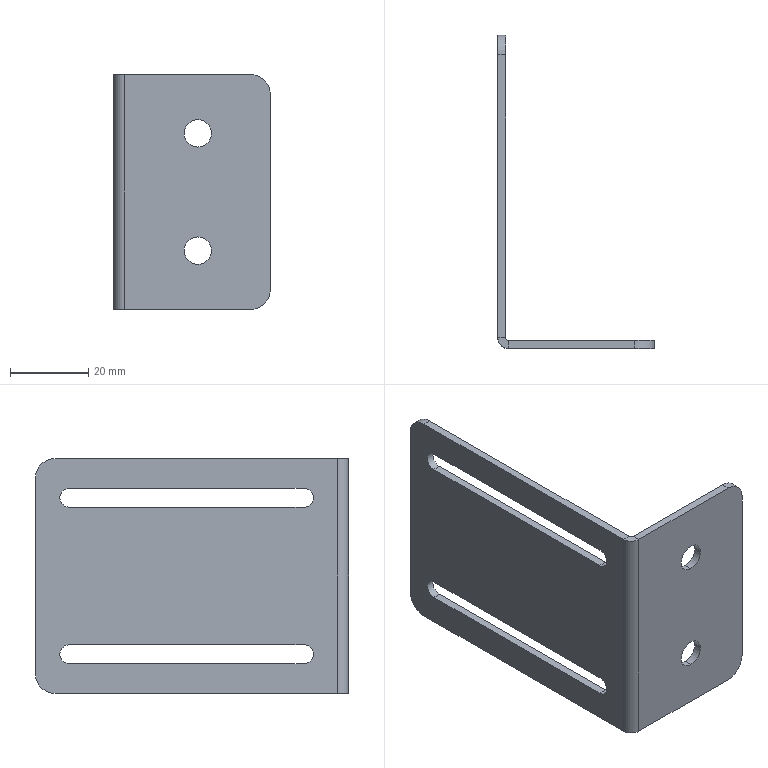Part | SolidWorks | features HoleWzd 2, BreakCorner 1, FlatPattern 1, SMBaseFlange 1, SheetMetal 1 | 1 solid | 30 faces | box 40 x 80 x 60 mm | volume 12649 mm3 | plane 16 | cylinder 14 | commonest cylinder face diameters 4.8 x4 7 x4 10 x4 1.473 x1 5.473 x1
STEP:
#1=CARTESIAN_POINT('',(21.5,0.,11.5));
#2=VERTEX_POINT('',#1);
#3=CARTESIAN_POINT('',(21.5,0.,18.5));
#4=VERTEX_POINT('',#3);
#5=CARTESIAN_POINT('',(21.5,0.,15.));
#6=DIRECTION('',(0.,1.,0.));
#7=DIRECTION('',(0.,0.,1.));
#8=AXIS2_PLACEMENT_3D('',#5,#6,#7);
#9=CIRCLE('',#8,3.5);
#10=EDGE_CURVE('',#2,#4,#9,.T.);
#11=ORIENTED_EDGE('',*,*,#10,.F.);
#12=CARTESIAN_POINT('',(21.5,2.,11.5));
#13=VERTEX_POINT('',#12);
#14=CARTESIAN_POINT('',(21.5,2.,11.5));
#15=DIRECTION('',(0.,1.,0.));
#16=VECTOR('',#15,1000.);
#17=LINE('',#14,#16);
#18=EDGE_CURVE('',#2,#13,#17,.T.);
#19=ORIENTED_EDGE('',*,*,#18,.T.);
#20=CARTESIAN_POINT('',(21.5,2.,18.5));
#21=VERTEX_POINT('',#20);
#22=CARTESIAN_POINT('',(21.5,2.,15.));
#23=DIRECTION('',(0.,1.,0.));
#24=DIRECTION('',(0.,0.,1.));
#25=AXIS2_PLACEMENT_3D('',#22,#23,#24);
#26=CIRCLE('',#25,3.5);
#27=EDGE_CURVE('',#13,#21,#26,.T.);
#28=ORIENTED_EDGE('',*,*,#27,.T.);
#29=CARTESIAN_POINT('',(21.5,2.,18.5));
#30=DIRECTION('',(0.,1.,0.));
#31=VECTOR('',#30,1000.);
#32=LINE('',#29,#31);
#33=EDGE_CURVE('',#4,#21,#32,.T.);
#34=ORIENTED_EDGE('',*,*,#33,.F.);
#35=EDGE_LOOP('',(#11,#19,#28,#34));
#36=FACE_OUTER_BOUND('',#35,.T.);
#37=CARTESIAN_POINT('',(21.5,2.,15.));
#38=DIRECTION('',(0.,1.,0.));
#39=DIRECTION('',(0.,0.,1.));
#40=AXIS2_PLACEMENT_3D('',#37,#38,#39);
#41=CYLINDRICAL_SURFACE('',#40,3.5);
#42=ADVANCED_FACE('',(#36),#41,.F.);
#43=CARTESIAN_POINT('',(21.5,0.,41.5));
#44=VERTEX_POINT('',#43);
#45=CARTESIAN_POINT('',(21.5,0.,48.5));
#46=VERTEX_POINT('',#45);
#47=CARTESIAN_POINT('',(21.5,0.,45.));
#48=DIRECTION('',(0.,1.,0.));
#49=DIRECTION('',(0.,0.,1.));
#50=AXIS2_PLACEMENT_3D('',#47,#48,#49);
#51=CIRCLE('',#50,3.5);
#52=EDGE_CURVE('',#44,#46,#51,.T.);
#53=ORIENTED_EDGE('',*,*,#52,.F.);
#54=CARTESIAN_POINT('',(21.5,2.,41.5));
#55=VERTEX_POINT('',#54);
#56=CARTESIAN_POINT('',(21.5,2.,41.5));
#57=DIRECTION('',(0.,1.,0.));
#58=VECTOR('',#57,1000.);
#59=LINE('',#56,#58);
#60=EDGE_CURVE('',#44,#55,#59,.T.);
#61=ORIENTED_EDGE('',*,*,#60,.T.);
#62=CARTESIAN_POINT('',(21.5,2.,48.5));
#63=VERTEX_POINT('',#62);
#64=CARTESIAN_POINT('',(21.5,2.,45.));
#65=DIRECTION('',(0.,1.,0.));
#66=DIRECTION('',(0.,0.,1.));
#67=AXIS2_PLACEMENT_3D('',#64,#65,#66);
#68=CIRCLE('',#67,3.5);
#69=EDGE_CURVE('',#55,#63,#68,.T.);
#70=ORIENTED_EDGE('',*,*,#69,.T.);
#71=CARTESIAN_POINT('',(21.5,2.,48.5));
#72=DIRECTION('',(0.,1.,0.));
#73=VECTOR('',#72,1000.);
#74=LINE('',#71,#73);
#75=EDGE_CURVE('',#46,#63,#74,.T.);
#76=ORIENTED_EDGE('',*,*,#75,.F.);
#77=EDGE_LOOP('',(#53,#61,#70,#76));
#78=FACE_OUTER_BOUND('',#77,.T.);
#79=CARTESIAN_POINT('',(21.5,2.,45.));
#80=DIRECTION('',(0.,1.,0.));
#81=DIRECTION('',(0.,0.,1.));
#82=AXIS2_PLACEMENT_3D('',#79,#80,#81);
#83=CYLINDRICAL_SURFACE('',#82,3.5);
#84=ADVANCED_FACE('',(#78),#83,.F.);
#85=CARTESIAN_POINT('',(2.,11.368,52.4));
#86=VERTEX_POINT('',#85);
#87=CARTESIAN_POINT('',(2.,11.368,47.6));
#88=VERTEX_POINT('',#87);
#89=CARTESIAN_POINT('',(2.,11.368,50.));
#90=DIRECTION('',(1.,0.,0.));
#91=DIRECTION('',(0.,0.,-1.));
#92=AXIS2_PLACEMENT_3D('',#89,#90,#91);
#93=CIRCLE('',#92,2.4);
#94=EDGE_CURVE('',#86,#88,#93,.T.);
#95=ORIENTED_EDGE('',*,*,#94,.F.);
#96=CARTESIAN_POINT('',(2.,71.368,52.4));
#97=VERTEX_POINT('',#96);
#98=CARTESIAN_POINT('',(2.,11.368,52.4));
#99=DIRECTION('',(0.,1.,0.));
#100=VECTOR('',#99,1000.);
#101=LINE('',#98,#100);
#102=EDGE_CURVE('',#86,#97,#101,.T.);
#103=ORIENTED_EDGE('',*,*,#102,.T.);
#104=CARTESIAN_POINT('',(2.,71.368,47.6));
#105=VERTEX_POINT('',#104);
#106=CARTESIAN_POINT('',(2.,71.368,50.));
#107=DIRECTION('',(1.,0.,0.));
#108=DIRECTION('',(0.,0.,-1.));
#109=AXIS2_PLACEMENT_3D('',#106,#107,#108);
#110=CIRCLE('',#109,2.4);
#111=EDGE_CURVE('',#105,#97,#110,.T.);
#112=ORIENTED_EDGE('',*,*,#111,.F.);
#113=CARTESIAN_POINT('',(2.,11.368,47.6));
#114=DIRECTION('',(0.,1.,0.));
#115=VECTOR('',#114,1000.);
#116=LINE('',#113,#115);
#117=EDGE_CURVE('',#88,#105,#116,.T.);
#118=ORIENTED_EDGE('',*,*,#117,.F.);
#119=EDGE_LOOP('',(#95,#103,#112,#118));
#120=FACE_BOUND('',#119,.T.);
#121=CARTESIAN_POINT('',(2.,80.,55.));
#122=VERTEX_POINT('',#121);
#123=CARTESIAN_POINT('',(2.,80.,5.));
#124=VERTEX_POINT('',#123);
#125=CARTESIAN_POINT('',(2.,80.,60.));
#126=DIRECTION('',(0.,0.,-1.));
#127=VECTOR('',#126,1000.);
#128=LINE('',#125,#127);
#129=EDGE_CURVE('',#122,#124,#128,.T.);
#130=ORIENTED_EDGE('',*,*,#129,.F.);
#131=CARTESIAN_POINT('',(2.,75.,60.));
#132=VERTEX_POINT('',#131);
#133=CARTESIAN_POINT('',(2.,75.,55.));
#134=DIRECTION('',(1.,0.,0.));
#135=DIRECTION('',(0.,0.,1.));
#136=AXIS2_PLACEMENT_3D('',#133,#134,#135);
#137=CIRCLE('',#136,5.);
#138=EDGE_CURVE('',#122,#132,#137,.T.);
#139=ORIENTED_EDGE('',*,*,#138,.T.);
#140=CARTESIAN_POINT('',(2.,2.737,60.));
#141=VERTEX_POINT('',#140);
#142=CARTESIAN_POINT('',(2.,0.,60.));
#143=DIRECTION('',(0.,1.,0.));
#144=VECTOR('',#143,1000.);
#145=LINE('',#142,#144);
#146=EDGE_CURVE('',#141,#132,#145,.T.);
#147=ORIENTED_EDGE('',*,*,#146,.F.);
#148=CARTESIAN_POINT('',(2.,2.737,0.));
#149=VERTEX_POINT('',#148);
#150=CARTESIAN_POINT('',(2.,2.737,60.));
#151=DIRECTION('',(0.,0.,-1.));
#152=VECTOR('',#151,1000.);
#153=LINE('',#150,#152);
#154=EDGE_CURVE('',#141,#149,#153,.T.);
#155=ORIENTED_EDGE('',*,*,#154,.T.);
#156=CARTESIAN_POINT('',(2.,75.,0.));
#157=VERTEX_POINT('',#156);
#158=CARTESIAN_POINT('',(2.,0.,0.));
#159=DIRECTION('',(0.,1.,0.));
#160=VECTOR('',#159,1000.);
#161=LINE('',#158,#160);
#162=EDGE_CURVE('',#149,#157,#161,.T.);
#163=ORIENTED_EDGE('',*,*,#162,.T.);
#164=CARTESIAN_POINT('',(2.,75.,5.));
#165=DIRECTION('',(1.,0.,0.));
#166=DIRECTION('',(0.,0.,1.));
#167=AXIS2_PLACEMENT_3D('',#164,#165,#166);
#168=CIRCLE('',#167,5.);
#169=EDGE_CURVE('',#157,#124,#168,.T.);
#170=ORIENTED_EDGE('',*,*,#169,.T.);
#171=EDGE_LOOP('',(#130,#139,#147,#155,#163,#170));
#172=FACE_OUTER_BOUND('',#171,.T.);
#173=CARTESIAN_POINT('',(2.,11.368,7.6));
#174=VERTEX_POINT('',#173);
#175=CARTESIAN_POINT('',(2.,71.368,7.6));
#176=VERTEX_POINT('',#175);
#177=CARTESIAN_POINT('',(2.,11.368,7.6));
#178=DIRECTION('',(0.,1.,0.));
#179=VECTOR('',#178,1000.);
#180=LINE('',#177,#179);
#181=EDGE_CURVE('',#174,#176,#180,.T.);
#182=ORIENTED_EDGE('',*,*,#181,.F.);
#183=CARTESIAN_POINT('',(2.,11.368,12.4));
#184=VERTEX_POINT('',#183);
#185=CARTESIAN_POINT('',(2.,11.368,10.));
#186=DIRECTION('',(1.,0.,0.));
#187=DIRECTION('',(0.,0.,-1.));
#188=AXIS2_PLACEMENT_3D('',#185,#186,#187);
#189=CIRCLE('',#188,2.4);
#190=EDGE_CURVE('',#184,#174,#189,.T.);
#191=ORIENTED_EDGE('',*,*,#190,.F.);
#192=CARTESIAN_POINT('',(2.,71.368,12.4));
#193=VERTEX_POINT('',#192);
#194=CARTESIAN_POINT('',(2.,11.368,12.4));
#195=DIRECTION('',(0.,1.,0.));
#196=VECTOR('',#195,1000.);
#197=LINE('',#194,#196);
#198=EDGE_CURVE('',#184,#193,#197,.T.);
#199=ORIENTED_EDGE('',*,*,#198,.T.);
#200=CARTESIAN_POINT('',(2.,71.368,10.));
#201=DIRECTION('',(1.,0.,0.));
#202=DIRECTION('',(0.,0.,-1.));
#203=AXIS2_PLACEMENT_3D('',#200,#201,#202);
#204=CIRCLE('',#203,2.4);
#205=EDGE_CURVE('',#176,#193,#204,.T.);
#206=ORIENTED_EDGE('',*,*,#205,.F.);
#207=EDGE_LOOP('',(#182,#191,#199,#206));
#208=FACE_BOUND('',#207,.T.);
#209=CARTESIAN_POINT('',(2.,0.,60.));
#210=DIRECTION('',(-1.,0.,0.));
#211=DIRECTION('',(0.,0.,1.));
#212=AXIS2_PLACEMENT_3D('',#209,#210,#211);
#213=PLANE('',#212);
#214=ADVANCED_FACE('',(#120,#172,#208),#213,.F.);
#215=CARTESIAN_POINT('',(0.,2.737,60.));
#216=VERTEX_POINT('',#215);
#217=CARTESIAN_POINT('',(0.,2.737,60.));
#218=DIRECTION('',(1.,0.,0.));
#219=VECTOR('',#218,1000.);
#220=LINE('',#217,#219);
#221=EDGE_CURVE('',#216,#141,#220,.T.);
#222=ORIENTED_EDGE('',*,*,#221,.F.);
#223=CARTESIAN_POINT('',(2.737,0.,60.));
#224=VERTEX_POINT('',#223);
#225=CARTESIAN_POINT('',(2.737,2.737,60.));
#226=DIRECTION('',(0.,0.,-1.));
#227=DIRECTION('',(1.,0.,0.));
#228=AXIS2_PLACEMENT_3D('',#225,#226,#227);
#229=CIRCLE('',#228,2.737);
#230=EDGE_CURVE('',#224,#216,#229,.T.);
#231=ORIENTED_EDGE('',*,*,#230,.F.);
#232=CARTESIAN_POINT('',(2.737,2.,60.));
#233=VERTEX_POINT('',#232);
#234=CARTESIAN_POINT('',(2.737,2.,60.));
#235=DIRECTION('',(0.,-1.,0.));
#236=VECTOR('',#235,1000.);
#237=LINE('',#234,#236);
#238=EDGE_CURVE('',#233,#224,#237,.T.);
#239=ORIENTED_EDGE('',*,*,#238,.F.);
#240=CARTESIAN_POINT('',(2.737,2.737,60.));
#241=DIRECTION('',(0.,0.,-1.));
#242=DIRECTION('',(1.,0.,0.));
#243=AXIS2_PLACEMENT_3D('',#240,#241,#242);
#244=CIRCLE('',#243,0.7366);
#245=EDGE_CURVE('',#233,#141,#244,.T.);
#246=ORIENTED_EDGE('',*,*,#245,.T.);
#247=EDGE_LOOP('',(#222,#231,#239,#246));
#248=FACE_OUTER_BOUND('',#247,.T.);
#249=CARTESIAN_POINT('',(0.,2.737,60.));
#250=DIRECTION('',(0.,0.,1.));
#251=DIRECTION('',(1.,0.,0.));
#252=AXIS2_PLACEMENT_3D('',#249,#250,#251);
#253=PLANE('',#252);
#254=ADVANCED_FACE('',(#248),#253,.T.);
#255=ORIENTED_EDGE('',*,*,#146,.T.);
#256=CARTESIAN_POINT('',(0.,75.,60.));
#257=VERTEX_POINT('',#256);
#258=CARTESIAN_POINT('',(2.737,75.,60.));
#259=DIRECTION('',(-1.,0.,0.));
#260=VECTOR('',#259,1000.);
#261=LINE('',#258,#260);
#262=EDGE_CURVE('',#132,#257,#261,.T.);
#263=ORIENTED_EDGE('',*,*,#262,.T.);
#264=CARTESIAN_POINT('',(0.,0.,60.));
#265=DIRECTION('',(0.,1.,0.));
#266=VECTOR('',#265,1000.);
#267=LINE('',#264,#266);
#268=EDGE_CURVE('',#216,#257,#267,.T.);
#269=ORIENTED_EDGE('',*,*,#268,.F.);
#270=ORIENTED_EDGE('',*,*,#221,.T.);
#271=EDGE_LOOP('',(#255,#263,#269,#270));
#272=FACE_OUTER_BOUND('',#271,.T.);
#273=CARTESIAN_POINT('',(2.737,2.,60.));
#274=DIRECTION('',(0.,0.,1.));
#275=DIRECTION('',(1.,0.,0.));
#276=AXIS2_PLACEMENT_3D('',#273,#274,#275);
#277=PLANE('',#276);
#278=ADVANCED_FACE('',(#272),#277,.T.);
#279=CARTESIAN_POINT('',(2.737,0.,0.));
#280=VERTEX_POINT('',#279);
#281=CARTESIAN_POINT('',(2.737,2.,0.));
#282=VERTEX_POINT('',#281);
#283=CARTESIAN_POINT('',(2.737,0.,0.));
#284=DIRECTION('',(0.,1.,0.));
#285=VECTOR('',#284,1000.);
#286=LINE('',#283,#285);
#287=EDGE_CURVE('',#280,#282,#286,.T.);
#288=ORIENTED_EDGE('',*,*,#287,.F.);
#289=CARTESIAN_POINT('',(0.,2.737,0.));
#290=VERTEX_POINT('',#289);
#291=CARTESIAN_POINT('',(2.737,2.737,0.));
#292=DIRECTION('',(0.,0.,-1.));
#293=DIRECTION('',(1.,0.,0.));
#294=AXIS2_PLACEMENT_3D('',#291,#292,#293);
#295=CIRCLE('',#294,2.737);
#296=EDGE_CURVE('',#280,#290,#295,.T.);
#297=ORIENTED_EDGE('',*,*,#296,.T.);
#298=CARTESIAN_POINT('',(2.,2.737,0.));
#299=DIRECTION('',(-1.,0.,0.));
#300=VECTOR('',#299,1000.);
#301=LINE('',#298,#300);
#302=EDGE_CURVE('',#149,#290,#301,.T.);
#303=ORIENTED_EDGE('',*,*,#302,.F.);
#304=CARTESIAN_POINT('',(2.737,2.737,0.));
#305=DIRECTION('',(0.,0.,-1.));
#306=DIRECTION('',(1.,0.,0.));
#307=AXIS2_PLACEMENT_3D('',#304,#305,#306);
#308=CIRCLE('',#307,0.7366);
#309=EDGE_CURVE('',#282,#149,#308,.T.);
#310=ORIENTED_EDGE('',*,*,#309,.F.);
#311=EDGE_LOOP('',(#288,#297,#303,#310));
#312=FACE_OUTER_BOUND('',#311,.T.);
#313=CARTESIAN_POINT('',(2.737,0.,0.));
#314=DIRECTION('',(0.,0.,-1.));
#315=DIRECTION('',(-1.,0.,0.));
#316=AXIS2_PLACEMENT_3D('',#313,#314,#315);
#317=PLANE('',#316);
#318=ADVANCED_FACE('',(#312),#317,.T.);
#319=CARTESIAN_POINT('',(35.,2.,0.));
#320=VERTEX_POINT('',#319);
#321=CARTESIAN_POINT('',(0.,2.,0.));
#322=DIRECTION('',(-1.,0.,0.));
#323=VECTOR('',#322,1000.);
#324=LINE('',#321,#323);
#325=EDGE_CURVE('',#320,#282,#324,.T.);
#326=ORIENTED_EDGE('',*,*,#325,.F.);
#327=CARTESIAN_POINT('',(35.,0.,0.));
#328=VERTEX_POINT('',#327);
#329=CARTESIAN_POINT('',(35.,2.737,0.));
#330=DIRECTION('',(0.,-1.,0.));
#331=VECTOR('',#330,1000.);
#332=LINE('',#329,#331);
#333=EDGE_CURVE('',#320,#328,#332,.T.);
#334=ORIENTED_EDGE('',*,*,#333,.T.);
#335=CARTESIAN_POINT('',(0.,0.,0.));
#336=DIRECTION('',(-1.,0.,0.));
#337=VECTOR('',#336,1000.);
#338=LINE('',#335,#337);
#339=EDGE_CURVE('',#328,#280,#338,.T.);
#340=ORIENTED_EDGE('',*,*,#339,.T.);
#341=ORIENTED_EDGE('',*,*,#287,.T.);
#342=EDGE_LOOP('',(#326,#334,#340,#341));
#343=FACE_OUTER_BOUND('',#342,.T.);
#344=CARTESIAN_POINT('',(2.,2.737,0.));
#345=DIRECTION('',(0.,0.,-1.));
#346=DIRECTION('',(-1.,0.,0.));
#347=AXIS2_PLACEMENT_3D('',#344,#345,#346);
#348=PLANE('',#347);
#349=ADVANCED_FACE('',(#343),#348,.T.);
#350=CARTESIAN_POINT('',(0.,80.,55.));
#351=VERTEX_POINT('',#350);
#352=CARTESIAN_POINT('',(0.,80.,5.));
#353=VERTEX_POINT('',#352);
#354=CARTESIAN_POINT('',(0.,80.,60.));
#355=DIRECTION('',(0.,0.,-1.));
#356=VECTOR('',#355,1000.);
#357=LINE('',#354,#356);
#358=EDGE_CURVE('',#351,#353,#357,.T.);
#359=ORIENTED_EDGE('',*,*,#358,.F.);
#360=CARTESIAN_POINT('',(0.,80.,55.));
#361=DIRECTION('',(1.,0.,0.));
#362=VECTOR('',#361,1000.);
#363=LINE('',#360,#362);
#364=EDGE_CURVE('',#351,#122,#363,.T.);
#365=ORIENTED_EDGE('',*,*,#364,.T.);
#366=ORIENTED_EDGE('',*,*,#129,.T.);
#367=CARTESIAN_POINT('',(0.,80.,5.));
#368=DIRECTION('',(-1.,0.,0.));
#369=VECTOR('',#368,1000.);
#370=LINE('',#367,#369);
#371=EDGE_CURVE('',#124,#353,#370,.T.);
#372=ORIENTED_EDGE('',*,*,#371,.T.);
#373=EDGE_LOOP('',(#359,#365,#366,#372));
#374=FACE_OUTER_BOUND('',#373,.T.);
#375=CARTESIAN_POINT('',(0.,80.,60.));
#376=DIRECTION('',(0.,1.,0.));
#377=DIRECTION('',(0.,0.,1.));
#378=AXIS2_PLACEMENT_3D('',#375,#376,#377);
#379=PLANE('',#378);
#380=ADVANCED_FACE('',(#374),#379,.T.);
#381=CARTESIAN_POINT('',(0.,11.368,52.4));
#382=VERTEX_POINT('',#381);
#383=CARTESIAN_POINT('',(0.,71.368,52.4));
#384=VERTEX_POINT('',#383);
#385=CARTESIAN_POINT('',(0.,11.368,52.4));
#386=DIRECTION('',(0.,1.,0.));
#387=VECTOR('',#386,1000.);
#388=LINE('',#385,#387);
#389=EDGE_CURVE('',#382,#384,#388,.T.);
#390=ORIENTED_EDGE('',*,*,#389,.F.);
#391=CARTESIAN_POINT('',(0.,11.368,47.6));
#392=VERTEX_POINT('',#391);
#393=CARTESIAN_POINT('',(0.,11.368,50.));
#394=DIRECTION('',(1.,0.,0.));
#395=DIRECTION('',(0.,0.,-1.));
#396=AXIS2_PLACEMENT_3D('',#393,#394,#395);
#397=CIRCLE('',#396,2.4);
#398=EDGE_CURVE('',#382,#392,#397,.T.);
#399=ORIENTED_EDGE('',*,*,#398,.T.);
#400=CARTESIAN_POINT('',(0.,71.368,47.6));
#401=VERTEX_POINT('',#400);
#402=CARTESIAN_POINT('',(0.,11.368,47.6));
#403=DIRECTION('',(0.,1.,0.));
#404=VECTOR('',#403,1000.);
#405=LINE('',#402,#404);
#406=EDGE_CURVE('',#392,#401,#405,.T.);
#407=ORIENTED_EDGE('',*,*,#406,.T.);
#408=CARTESIAN_POINT('',(0.,71.368,50.));
#409=DIRECTION('',(1.,0.,0.));
#410=DIRECTION('',(0.,0.,-1.));
#411=AXIS2_PLACEMENT_3D('',#408,#409,#410);
#412=CIRCLE('',#411,2.4);
#413=EDGE_CURVE('',#401,#384,#412,.T.);
#414=ORIENTED_EDGE('',*,*,#413,.T.);
#415=EDGE_LOOP('',(#390,#399,#407,#414));
#416=FACE_BOUND('',#415,.T.);
#417=CARTESIAN_POINT('',(0.,11.368,12.4));
#418=VERTEX_POINT('',#417);
#419=CARTESIAN_POINT('',(0.,11.368,7.6));
#420=VERTEX_POINT('',#419);
#421=CARTESIAN_POINT('',(0.,11.368,10.));
#422=DIRECTION('',(1.,0.,0.));
#423=DIRECTION('',(0.,0.,-1.));
#424=AXIS2_PLACEMENT_3D('',#421,#422,#423);
#425=CIRCLE('',#424,2.4);
#426=EDGE_CURVE('',#418,#420,#425,.T.);
#427=ORIENTED_EDGE('',*,*,#426,.T.);
#428=CARTESIAN_POINT('',(0.,71.368,7.6));
#429=VERTEX_POINT('',#428);
#430=CARTESIAN_POINT('',(0.,11.368,7.6));
#431=DIRECTION('',(0.,1.,0.));
#432=VECTOR('',#431,1000.);
#433=LINE('',#430,#432);
#434=EDGE_CURVE('',#420,#429,#433,.T.);
#435=ORIENTED_EDGE('',*,*,#434,.T.);
#436=CARTESIAN_POINT('',(0.,71.368,12.4));
#437=VERTEX_POINT('',#436);
#438=CARTESIAN_POINT('',(0.,71.368,10.));
#439=DIRECTION('',(1.,0.,0.));
#440=DIRECTION('',(0.,0.,-1.));
#441=AXIS2_PLACEMENT_3D('',#438,#439,#440);
#442=CIRCLE('',#441,2.4);
#443=EDGE_CURVE('',#429,#437,#442,.T.);
#444=ORIENTED_EDGE('',*,*,#443,.T.);
#445=CARTESIAN_POINT('',(0.,11.368,12.4));
#446=DIRECTION('',(0.,1.,0.));
#447=VECTOR('',#446,1000.);
#448=LINE('',#445,#447);
#449=EDGE_CURVE('',#418,#437,#448,.T.);
#450=ORIENTED_EDGE('',*,*,#449,.F.);
#451=EDGE_LOOP('',(#427,#435,#444,#450));
#452=FACE_BOUND('',#451,.T.);
#453=ORIENTED_EDGE('',*,*,#268,.T.);
#454=CARTESIAN_POINT('',(0.,75.,55.));
#455=DIRECTION('',(-1.,0.,0.));
#456=DIRECTION('',(0.,0.,1.));
#457=AXIS2_PLACEMENT_3D('',#454,#455,#456);
#458=CIRCLE('',#457,5.);
#459=EDGE_CURVE('',#257,#351,#458,.T.);
#460=ORIENTED_EDGE('',*,*,#459,.T.);
#461=ORIENTED_EDGE('',*,*,#358,.T.);
#462=CARTESIAN_POINT('',(0.,75.,0.));
#463=VERTEX_POINT('',#462);
#464=CARTESIAN_POINT('',(0.,75.,5.));
#465=DIRECTION('',(-1.,0.,0.));
#466=DIRECTION('',(0.,0.,1.));
#467=AXIS2_PLACEMENT_3D('',#464,#465,#466);
#468=CIRCLE('',#467,5.);
#469=EDGE_CURVE('',#353,#463,#468,.T.);
#470=ORIENTED_EDGE('',*,*,#469,.T.);
#471=CARTESIAN_POINT('',(0.,0.,0.));
#472=DIRECTION('',(0.,1.,0.));
#473=VECTOR('',#472,1000.);
#474=LINE('',#471,#473);
#475=EDGE_CURVE('',#290,#463,#474,.T.);
#476=ORIENTED_EDGE('',*,*,#475,.F.);
#477=CARTESIAN_POINT('',(0.,2.737,60.));
#478=DIRECTION('',(0.,0.,-1.));
#479=VECTOR('',#478,1000.);
#480=LINE('',#477,#479);
#481=EDGE_CURVE('',#216,#290,#480,.T.);
#482=ORIENTED_EDGE('',*,*,#481,.F.);
#483=EDGE_LOOP('',(#453,#460,#461,#470,#476,#482));
#484=FACE_OUTER_BOUND('',#483,.T.);
#485=CARTESIAN_POINT('',(0.,0.,60.));
#486=DIRECTION('',(-1.,0.,0.));
#487=DIRECTION('',(0.,0.,1.));
#488=AXIS2_PLACEMENT_3D('',#485,#486,#487);
#489=PLANE('',#488);
#490=ADVANCED_FACE('',(#416,#452,#484),#489,.T.);
#491=ORIENTED_EDGE('',*,*,#296,.F.);
#492=CARTESIAN_POINT('',(2.737,0.,60.));
#493=DIRECTION('',(0.,0.,-1.));
#494=VECTOR('',#493,1000.);
#495=LINE('',#492,#494);
#496=EDGE_CURVE('',#224,#280,#495,.T.);
#497=ORIENTED_EDGE('',*,*,#496,.F.);
#498=ORIENTED_EDGE('',*,*,#230,.T.);
#499=ORIENTED_EDGE('',*,*,#481,.T.);
#500=EDGE_LOOP('',(#491,#497,#498,#499));
#501=FACE_OUTER_BOUND('',#500,.T.);
#502=CARTESIAN_POINT('',(2.737,2.737,60.));
#503=DIRECTION('',(0.,0.,-1.));
#504=DIRECTION('',(-1.,0.,0.));
#505=AXIS2_PLACEMENT_3D('',#502,#503,#504);
#506=CYLINDRICAL_SURFACE('',#505,2.737);
#507=ADVANCED_FACE('',(#501),#506,.T.);
#508=CARTESIAN_POINT('',(21.5,0.,15.));
#509=DIRECTION('',(0.,1.,0.));
#510=DIRECTION('',(0.,0.,1.));
#511=AXIS2_PLACEMENT_3D('',#508,#509,#510);
#512=CIRCLE('',#511,3.5);
#513=EDGE_CURVE('',#4,#2,#512,.T.);
#514=ORIENTED_EDGE('',*,*,#513,.T.);
#515=ORIENTED_EDGE('',*,*,#10,.T.);
#516=EDGE_LOOP('',(#514,#515));
#517=FACE_BOUND('',#516,.T.);
#518=CARTESIAN_POINT('',(21.5,0.,45.));
#519=DIRECTION('',(0.,1.,0.));
#520=DIRECTION('',(0.,0.,1.));
#521=AXIS2_PLACEMENT_3D('',#518,#519,#520);
#522=CIRCLE('',#521,3.5);
#523=EDGE_CURVE('',#46,#44,#522,.T.);
#524=ORIENTED_EDGE('',*,*,#523,.T.);
#525=ORIENTED_EDGE('',*,*,#52,.T.);
#526=EDGE_LOOP('',(#524,#525));
#527=FACE_BOUND('',#526,.T.);
#528=CARTESIAN_POINT('',(40.,0.,55.));
#529=VERTEX_POINT('',#528);
#530=CARTESIAN_POINT('',(40.,0.,5.));
#531=VERTEX_POINT('',#530);
#532=CARTESIAN_POINT('',(40.,0.,60.));
#533=DIRECTION('',(0.,0.,-1.));
#534=VECTOR('',#533,1000.);
#535=LINE('',#532,#534);
#536=EDGE_CURVE('',#529,#531,#535,.T.);
#537=ORIENTED_EDGE('',*,*,#536,.F.);
#538=CARTESIAN_POINT('',(35.,0.,60.));
#539=VERTEX_POINT('',#538);
#540=CARTESIAN_POINT('',(35.,0.,55.));
#541=DIRECTION('',(0.,-1.,0.));
#542=DIRECTION('',(0.,0.,-1.));
#543=AXIS2_PLACEMENT_3D('',#540,#541,#542);
#544=CIRCLE('',#543,5.);
#545=EDGE_CURVE('',#529,#539,#544,.T.);
#546=ORIENTED_EDGE('',*,*,#545,.T.);
#547=CARTESIAN_POINT('',(0.,0.,60.));
#548=DIRECTION('',(-1.,0.,0.));
#549=VECTOR('',#548,1000.);
#550=LINE('',#547,#549);
#551=EDGE_CURVE('',#539,#224,#550,.T.);
#552=ORIENTED_EDGE('',*,*,#551,.T.);
#553=ORIENTED_EDGE('',*,*,#496,.T.);
#554=ORIENTED_EDGE('',*,*,#339,.F.);
#555=CARTESIAN_POINT('',(35.,0.,5.));
#556=DIRECTION('',(0.,-1.,0.));
#557=DIRECTION('',(0.,0.,-1.));
#558=AXIS2_PLACEMENT_3D('',#555,#556,#557);
#559=CIRCLE('',#558,5.);
#560=EDGE_CURVE('',#328,#531,#559,.T.);
#561=ORIENTED_EDGE('',*,*,#560,.T.);
#562=EDGE_LOOP('',(#537,#546,#552,#553,#554,#561));
#563=FACE_OUTER_BOUND('',#562,.T.);
#564=CARTESIAN_POINT('',(0.,0.,60.));
#565=DIRECTION('',(0.,-1.,0.));
#566=DIRECTION('',(0.,0.,-1.));
#567=AXIS2_PLACEMENT_3D('',#564,#565,#566);
#568=PLANE('',#567);
#569=ADVANCED_FACE('',(#517,#527,#563),#568,.T.);
#570=CARTESIAN_POINT('',(40.,2.,55.));
#571=VERTEX_POINT('',#570);
#572=CARTESIAN_POINT('',(40.,2.,5.));
#573=VERTEX_POINT('',#572);
#574=CARTESIAN_POINT('',(40.,2.,60.));
#575=DIRECTION('',(0.,0.,-1.));
#576=VECTOR('',#575,1000.);
#577=LINE('',#574,#576);
#578=EDGE_CURVE('',#571,#573,#577,.T.);
#579=ORIENTED_EDGE('',*,*,#578,.F.);
#580=CARTESIAN_POINT('',(40.,2.,55.));
#581=DIRECTION('',(0.,-1.,0.));
#582=VECTOR('',#581,1000.);
#583=LINE('',#580,#582);
#584=EDGE_CURVE('',#571,#529,#583,.T.);
#585=ORIENTED_EDGE('',*,*,#584,.T.);
#586=ORIENTED_EDGE('',*,*,#536,.T.);
#587=CARTESIAN_POINT('',(40.,2.,5.));
#588=DIRECTION('',(0.,1.,0.));
#589=VECTOR('',#588,1000.);
#590=LINE('',#587,#589);
#591=EDGE_CURVE('',#531,#573,#590,.T.);
#592=ORIENTED_EDGE('',*,*,#591,.T.);
#593=EDGE_LOOP('',(#579,#585,#586,#592));
#594=FACE_OUTER_BOUND('',#593,.T.);
#595=CARTESIAN_POINT('',(40.,2.,60.));
#596=DIRECTION('',(1.,0.,0.));
#597=DIRECTION('',(0.,0.,-1.));
#598=AXIS2_PLACEMENT_3D('',#595,#596,#597);
#599=PLANE('',#598);
#600=ADVANCED_FACE('',(#594),#599,.T.);
#601=CARTESIAN_POINT('',(21.5,2.,15.));
#602=DIRECTION('',(0.,1.,0.));
#603=DIRECTION('',(0.,0.,1.));
#604=AXIS2_PLACEMENT_3D('',#601,#602,#603);
#605=CIRCLE('',#604,3.5);
#606=EDGE_CURVE('',#21,#13,#605,.T.);
#607=ORIENTED_EDGE('',*,*,#606,.F.);
#608=ORIENTED_EDGE('',*,*,#27,.F.);
#609=EDGE_LOOP('',(#607,#608));
#610=FACE_BOUND('',#609,.T.);
#611=CARTESIAN_POINT('',(21.5,2.,45.));
#612=DIRECTION('',(0.,1.,0.));
#613=DIRECTION('',(0.,0.,1.));
#614=AXIS2_PLACEMENT_3D('',#611,#612,#613);
#615=CIRCLE('',#614,3.5);
#616=EDGE_CURVE('',#63,#55,#615,.T.);
#617=ORIENTED_EDGE('',*,*,#616,.F.);
#618=ORIENTED_EDGE('',*,*,#69,.F.);
#619=EDGE_LOOP('',(#617,#618));
#620=FACE_BOUND('',#619,.T.);
#621=CARTESIAN_POINT('',(35.,2.,60.));
#622=VERTEX_POINT('',#621);
#623=CARTESIAN_POINT('',(0.,2.,60.));
#624=DIRECTION('',(-1.,0.,0.));
#625=VECTOR('',#624,1000.);
#626=LINE('',#623,#625);
#627=EDGE_CURVE('',#622,#233,#626,.T.);
#628=ORIENTED_EDGE('',*,*,#627,.F.);
#629=CARTESIAN_POINT('',(35.,2.,55.));
#630=DIRECTION('',(0.,1.,0.));
#631=DIRECTION('',(0.,0.,-1.));
#632=AXIS2_PLACEMENT_3D('',#629,#630,#631);
#633=CIRCLE('',#632,5.);
#634=EDGE_CURVE('',#622,#571,#633,.T.);
#635=ORIENTED_EDGE('',*,*,#634,.T.);
#636=ORIENTED_EDGE('',*,*,#578,.T.);
#637=CARTESIAN_POINT('',(35.,2.,5.));
#638=DIRECTION('',(0.,1.,0.));
#639=DIRECTION('',(0.,0.,-1.));
#640=AXIS2_PLACEMENT_3D('',#637,#638,#639);
#641=CIRCLE('',#640,5.);
#642=EDGE_CURVE('',#573,#320,#641,.T.);
#643=ORIENTED_EDGE('',*,*,#642,.T.);
#644=ORIENTED_EDGE('',*,*,#325,.T.);
#645=CARTESIAN_POINT('',(2.737,2.,60.));
#646=DIRECTION('',(0.,0.,-1.));
#647=VECTOR('',#646,1000.);
#648=LINE('',#645,#647);
#649=EDGE_CURVE('',#233,#282,#648,.T.);
#650=ORIENTED_EDGE('',*,*,#649,.F.);
#651=EDGE_LOOP('',(#628,#635,#636,#643,#644,#650));
#652=FACE_OUTER_BOUND('',#651,.T.);
#653=CARTESIAN_POINT('',(0.,2.,60.));
#654=DIRECTION('',(0.,-1.,0.));
#655=DIRECTION('',(0.,0.,-1.));
#656=AXIS2_PLACEMENT_3D('',#653,#654,#655);
#657=PLANE('',#656);
#658=ADVANCED_FACE('',(#610,#620,#652),#657,.F.);
#659=ORIENTED_EDGE('',*,*,#309,.T.);
#660=ORIENTED_EDGE('',*,*,#154,.F.);
#661=ORIENTED_EDGE('',*,*,#245,.F.);
#662=ORIENTED_EDGE('',*,*,#649,.T.);
#663=EDGE_LOOP('',(#659,#660,#661,#662));
#664=FACE_OUTER_BOUND('',#663,.T.);
#665=CARTESIAN_POINT('',(2.737,2.737,60.));
#666=DIRECTION('',(0.,0.,-1.));
#667=DIRECTION('',(-1.,0.,0.));
#668=AXIS2_PLACEMENT_3D('',#665,#666,#667);
#669=CYLINDRICAL_SURFACE('',#668,0.7366);
#670=ADVANCED_FACE('',(#664),#669,.F.);
#671=ORIENTED_EDGE('',*,*,#551,.F.);
#672=CARTESIAN_POINT('',(35.,2.737,60.));
#673=DIRECTION('',(0.,1.,0.));
#674=VECTOR('',#673,1000.);
#675=LINE('',#672,#674);
#676=EDGE_CURVE('',#539,#622,#675,.T.);
#677=ORIENTED_EDGE('',*,*,#676,.T.);
#678=ORIENTED_EDGE('',*,*,#627,.T.);
#679=ORIENTED_EDGE('',*,*,#238,.T.);
#680=EDGE_LOOP('',(#671,#677,#678,#679));
#681=FACE_OUTER_BOUND('',#680,.T.);
#682=CARTESIAN_POINT('',(2.737,2.737,60.));
#683=DIRECTION('',(0.,0.,1.));
#684=DIRECTION('',(1.,0.,0.));
#685=AXIS2_PLACEMENT_3D('',#682,#683,#684);
#686=PLANE('',#685);
#687=ADVANCED_FACE('',(#681),#686,.T.);
#688=ORIENTED_EDGE('',*,*,#475,.T.);
#689=CARTESIAN_POINT('',(2.,75.,0.));
#690=DIRECTION('',(1.,0.,0.));
#691=VECTOR('',#690,1000.);
#692=LINE('',#689,#691);
#693=EDGE_CURVE('',#463,#157,#692,.T.);
#694=ORIENTED_EDGE('',*,*,#693,.T.);
#695=ORIENTED_EDGE('',*,*,#162,.F.);
#696=ORIENTED_EDGE('',*,*,#302,.T.);
#697=EDGE_LOOP('',(#688,#694,#695,#696));
#698=FACE_OUTER_BOUND('',#697,.T.);
#699=CARTESIAN_POINT('',(2.737,2.737,0.));
#700=DIRECTION('',(0.,0.,1.));
#701=DIRECTION('',(1.,0.,0.));
#702=AXIS2_PLACEMENT_3D('',#699,#700,#701);
#703=PLANE('',#702);
#704=ADVANCED_FACE('',(#698),#703,.F.);
#705=ORIENTED_EDGE('',*,*,#443,.F.);
#706=CARTESIAN_POINT('',(2.,71.368,7.6));
#707=DIRECTION('',(-1.,0.,0.));
#708=VECTOR('',#707,1000.);
#709=LINE('',#706,#708);
#710=EDGE_CURVE('',#176,#429,#709,.T.);
#711=ORIENTED_EDGE('',*,*,#710,.F.);
#712=ORIENTED_EDGE('',*,*,#205,.T.);
#713=CARTESIAN_POINT('',(2.,71.368,12.4));
#714=DIRECTION('',(1.,0.,0.));
#715=VECTOR('',#714,1000.);
#716=LINE('',#713,#715);
#717=EDGE_CURVE('',#437,#193,#716,.T.);
#718=ORIENTED_EDGE('',*,*,#717,.F.);
#719=EDGE_LOOP('',(#705,#711,#712,#718));
#720=FACE_OUTER_BOUND('',#719,.T.);
#721=CARTESIAN_POINT('',(2.,71.368,10.));
#722=DIRECTION('',(1.,0.,0.));
#723=DIRECTION('',(0.,0.,-1.));
#724=AXIS2_PLACEMENT_3D('',#721,#722,#723);
#725=CYLINDRICAL_SURFACE('',#724,2.4);
#726=ADVANCED_FACE('',(#720),#725,.F.);
#727=ORIENTED_EDGE('',*,*,#190,.T.);
#728=CARTESIAN_POINT('',(2.,11.368,7.6));
#729=DIRECTION('',(1.,0.,0.));
#730=VECTOR('',#729,1000.);
#731=LINE('',#728,#730);
#732=EDGE_CURVE('',#420,#174,#731,.T.);
#733=ORIENTED_EDGE('',*,*,#732,.F.);
#734=ORIENTED_EDGE('',*,*,#426,.F.);
#735=CARTESIAN_POINT('',(2.,11.368,12.4));
#736=DIRECTION('',(-1.,0.,0.));
#737=VECTOR('',#736,1000.);
#738=LINE('',#735,#737);
#739=EDGE_CURVE('',#184,#418,#738,.T.);
#740=ORIENTED_EDGE('',*,*,#739,.F.);
#741=EDGE_LOOP('',(#727,#733,#734,#740));
#742=FACE_OUTER_BOUND('',#741,.T.);
#743=CARTESIAN_POINT('',(2.,11.368,10.));
#744=DIRECTION('',(1.,0.,0.));
#745=DIRECTION('',(0.,0.,-1.));
#746=AXIS2_PLACEMENT_3D('',#743,#744,#745);
#747=CYLINDRICAL_SURFACE('',#746,2.4);
#748=ADVANCED_FACE('',(#742),#747,.F.);
#749=ORIENTED_EDGE('',*,*,#717,.T.);
#750=ORIENTED_EDGE('',*,*,#198,.F.);
#751=ORIENTED_EDGE('',*,*,#739,.T.);
#752=ORIENTED_EDGE('',*,*,#449,.T.);
#753=EDGE_LOOP('',(#749,#750,#751,#752));
#754=FACE_OUTER_BOUND('',#753,.T.);
#755=CARTESIAN_POINT('',(2.,11.368,12.4));
#756=DIRECTION('',(0.,0.,1.));
#757=DIRECTION('',(1.,0.,0.));
#758=AXIS2_PLACEMENT_3D('',#755,#756,#757);
#759=PLANE('',#758);
#760=ADVANCED_FACE('',(#754),#759,.F.);
#761=ORIENTED_EDGE('',*,*,#710,.T.);
#762=ORIENTED_EDGE('',*,*,#434,.F.);
#763=ORIENTED_EDGE('',*,*,#732,.T.);
#764=ORIENTED_EDGE('',*,*,#181,.T.);
#765=EDGE_LOOP('',(#761,#762,#763,#764));
#766=FACE_OUTER_BOUND('',#765,.T.);
#767=CARTESIAN_POINT('',(2.,11.368,7.6));
#768=DIRECTION('',(0.,0.,-1.));
#769=DIRECTION('',(-1.,0.,0.));
#770=AXIS2_PLACEMENT_3D('',#767,#768,#769);
#771=PLANE('',#770);
#772=ADVANCED_FACE('',(#766),#771,.F.);
#773=ORIENTED_EDGE('',*,*,#413,.F.);
#774=CARTESIAN_POINT('',(2.,71.368,47.6));
#775=DIRECTION('',(-1.,0.,0.));
#776=VECTOR('',#775,1000.);
#777=LINE('',#774,#776);
#778=EDGE_CURVE('',#105,#401,#777,.T.);
#779=ORIENTED_EDGE('',*,*,#778,.F.);
#780=ORIENTED_EDGE('',*,*,#111,.T.);
#781=CARTESIAN_POINT('',(2.,71.368,52.4));
#782=DIRECTION('',(1.,0.,0.));
#783=VECTOR('',#782,1000.);
#784=LINE('',#781,#783);
#785=EDGE_CURVE('',#384,#97,#784,.T.);
#786=ORIENTED_EDGE('',*,*,#785,.F.);
#787=EDGE_LOOP('',(#773,#779,#780,#786));
#788=FACE_OUTER_BOUND('',#787,.T.);
#789=CARTESIAN_POINT('',(2.,71.368,50.));
#790=DIRECTION('',(1.,0.,0.));
#791=DIRECTION('',(0.,0.,-1.));
#792=AXIS2_PLACEMENT_3D('',#789,#790,#791);
#793=CYLINDRICAL_SURFACE('',#792,2.4);
#794=ADVANCED_FACE('',(#788),#793,.F.);
#795=ORIENTED_EDGE('',*,*,#94,.T.);
#796=CARTESIAN_POINT('',(2.,11.368,47.6));
#797=DIRECTION('',(1.,0.,0.));
#798=VECTOR('',#797,1000.);
#799=LINE('',#796,#798);
#800=EDGE_CURVE('',#392,#88,#799,.T.);
#801=ORIENTED_EDGE('',*,*,#800,.F.);
#802=ORIENTED_EDGE('',*,*,#398,.F.);
#803=CARTESIAN_POINT('',(2.,11.368,52.4));
#804=DIRECTION('',(-1.,0.,0.));
#805=VECTOR('',#804,1000.);
#806=LINE('',#803,#805);
#807=EDGE_CURVE('',#86,#382,#806,.T.);
#808=ORIENTED_EDGE('',*,*,#807,.F.);
#809=EDGE_LOOP('',(#795,#801,#802,#808));
#810=FACE_OUTER_BOUND('',#809,.T.);
#811=CARTESIAN_POINT('',(2.,11.368,50.));
#812=DIRECTION('',(1.,0.,0.));
#813=DIRECTION('',(0.,0.,-1.));
#814=AXIS2_PLACEMENT_3D('',#811,#812,#813);
#815=CYLINDRICAL_SURFACE('',#814,2.4);
#816=ADVANCED_FACE('',(#810),#815,.F.);
#817=ORIENTED_EDGE('',*,*,#785,.T.);
#818=ORIENTED_EDGE('',*,*,#102,.F.);
#819=ORIENTED_EDGE('',*,*,#807,.T.);
#820=ORIENTED_EDGE('',*,*,#389,.T.);
#821=EDGE_LOOP('',(#817,#818,#819,#820));
#822=FACE_OUTER_BOUND('',#821,.T.);
#823=CARTESIAN_POINT('',(2.,11.368,52.4));
#824=DIRECTION('',(0.,0.,1.));
#825=DIRECTION('',(1.,0.,0.));
#826=AXIS2_PLACEMENT_3D('',#823,#824,#825);
#827=PLANE('',#826);
#828=ADVANCED_FACE('',(#822),#827,.F.);
#829=ORIENTED_EDGE('',*,*,#778,.T.);
#830=ORIENTED_EDGE('',*,*,#406,.F.);
#831=ORIENTED_EDGE('',*,*,#800,.T.);
#832=ORIENTED_EDGE('',*,*,#117,.T.);
#833=EDGE_LOOP('',(#829,#830,#831,#832));
#834=FACE_OUTER_BOUND('',#833,.T.);
#835=CARTESIAN_POINT('',(2.,11.368,47.6));
#836=DIRECTION('',(0.,0.,-1.));
#837=DIRECTION('',(-1.,0.,0.));
#838=AXIS2_PLACEMENT_3D('',#835,#836,#837);
#839=PLANE('',#838);
#840=ADVANCED_FACE('',(#834),#839,.F.);
#841=ORIENTED_EDGE('',*,*,#60,.F.);
#842=ORIENTED_EDGE('',*,*,#523,.F.);
#843=ORIENTED_EDGE('',*,*,#75,.T.);
#844=ORIENTED_EDGE('',*,*,#616,.T.);
#845=EDGE_LOOP('',(#841,#842,#843,#844));
#846=FACE_OUTER_BOUND('',#845,.T.);
#847=CARTESIAN_POINT('',(21.5,2.,45.));
#848=DIRECTION('',(0.,1.,0.));
#849=DIRECTION('',(0.,0.,1.));
#850=AXIS2_PLACEMENT_3D('',#847,#848,#849);
#851=CYLINDRICAL_SURFACE('',#850,3.5);
#852=ADVANCED_FACE('',(#846),#851,.F.);
#853=ORIENTED_EDGE('',*,*,#18,.F.);
#854=ORIENTED_EDGE('',*,*,#513,.F.);
#855=ORIENTED_EDGE('',*,*,#33,.T.);
#856=ORIENTED_EDGE('',*,*,#606,.T.);
#857=EDGE_LOOP('',(#853,#854,#855,#856));
#858=FACE_OUTER_BOUND('',#857,.T.);
#859=CARTESIAN_POINT('',(21.5,2.,15.));
#860=DIRECTION('',(0.,1.,0.));
#861=DIRECTION('',(0.,0.,1.));
#862=AXIS2_PLACEMENT_3D('',#859,#860,#861);
#863=CYLINDRICAL_SURFACE('',#862,3.5);
#864=ADVANCED_FACE('',(#858),#863,.F.);
#865=ORIENTED_EDGE('',*,*,#634,.F.);
#866=ORIENTED_EDGE('',*,*,#676,.F.);
#867=ORIENTED_EDGE('',*,*,#545,.F.);
#868=ORIENTED_EDGE('',*,*,#584,.F.);
#869=EDGE_LOOP('',(#865,#866,#867,#868));
#870=FACE_OUTER_BOUND('',#869,.T.);
#871=CARTESIAN_POINT('',(35.,2.,55.));
#872=DIRECTION('',(0.,-1.,0.));
#873=DIRECTION('',(0.,0.,-1.));
#874=AXIS2_PLACEMENT_3D('',#871,#872,#873);
#875=CYLINDRICAL_SURFACE('',#874,5.);
#876=ADVANCED_FACE('',(#870),#875,.T.);
#877=ORIENTED_EDGE('',*,*,#642,.F.);
#878=ORIENTED_EDGE('',*,*,#591,.F.);
#879=ORIENTED_EDGE('',*,*,#560,.F.);
#880=ORIENTED_EDGE('',*,*,#333,.F.);
#881=EDGE_LOOP('',(#877,#878,#879,#880));
#882=FACE_OUTER_BOUND('',#881,.T.);
#883=CARTESIAN_POINT('',(35.,2.737,5.));
#884=DIRECTION('',(0.,-1.,0.));
#885=DIRECTION('',(0.,0.,-1.));
#886=AXIS2_PLACEMENT_3D('',#883,#884,#885);
#887=CYLINDRICAL_SURFACE('',#886,5.);
#888=ADVANCED_FACE('',(#882),#887,.T.);
#889=ORIENTED_EDGE('',*,*,#459,.F.);
#890=ORIENTED_EDGE('',*,*,#262,.F.);
#891=ORIENTED_EDGE('',*,*,#138,.F.);
#892=ORIENTED_EDGE('',*,*,#364,.F.);
#893=EDGE_LOOP('',(#889,#890,#891,#892));
#894=FACE_OUTER_BOUND('',#893,.T.);
#895=CARTESIAN_POINT('',(0.,75.,55.));
#896=DIRECTION('',(1.,0.,0.));
#897=DIRECTION('',(0.,0.,-1.));
#898=AXIS2_PLACEMENT_3D('',#895,#896,#897);
#899=CYLINDRICAL_SURFACE('',#898,5.);
#900=ADVANCED_FACE('',(#894),#899,.T.);
#901=ORIENTED_EDGE('',*,*,#469,.F.);
#902=ORIENTED_EDGE('',*,*,#371,.F.);
#903=ORIENTED_EDGE('',*,*,#169,.F.);
#904=ORIENTED_EDGE('',*,*,#693,.F.);
#905=EDGE_LOOP('',(#901,#902,#903,#904));
#906=FACE_OUTER_BOUND('',#905,.T.);
#907=CARTESIAN_POINT('',(2.737,75.,5.));
#908=DIRECTION('',(-1.,0.,0.));
#909=DIRECTION('',(0.,0.,1.));
#910=AXIS2_PLACEMENT_3D('',#907,#908,#909);
#911=CYLINDRICAL_SURFACE('',#910,5.);
#912=ADVANCED_FACE('',(#906),#911,.T.);
#913=CLOSED_SHELL('',(#42,#84,#214,#254,#278,#318,#349,#380,#490,#507,#569,#600,#658,#670,#687,#704,#726,#748,#760,#772,#794,#816,#828,#840,#852,#864,#876,#888,#900,#912));
#914=MANIFOLD_SOLID_BREP('',#913);
#915=CARTESIAN_POINT('',(0.,0.,0.));
#916=DIRECTION('',(0.,0.,1.));
#917=DIRECTION('',(1.,0.,0.));
#918=AXIS2_PLACEMENT_3D('',#915,#916,#917);
#919=(LENGTH_UNIT()NAMED_UNIT(*)SI_UNIT(.MILLI.,.METRE.));
#920=UNCERTAINTY_MEASURE_WITH_UNIT(LENGTH_MEASURE(0.00001),#919,'','');
#921=(NAMED_UNIT(*)PLANE_ANGLE_UNIT()SI_UNIT($,.RADIAN.));
#922=(NAMED_UNIT(*)SI_UNIT($,.STERADIAN.)SOLID_ANGLE_UNIT());
#923=(GEOMETRIC_REPRESENTATION_CONTEXT(3)GLOBAL_UNCERTAINTY_ASSIGNED_CONTEXT((#920))GLOBAL_UNIT_ASSIGNED_CONTEXT((#919,#921,#922))REPRESENTATION_CONTEXT('',''));
#924=ADVANCED_BREP_SHAPE_REPRESENTATION('',(#914,#918),#923);